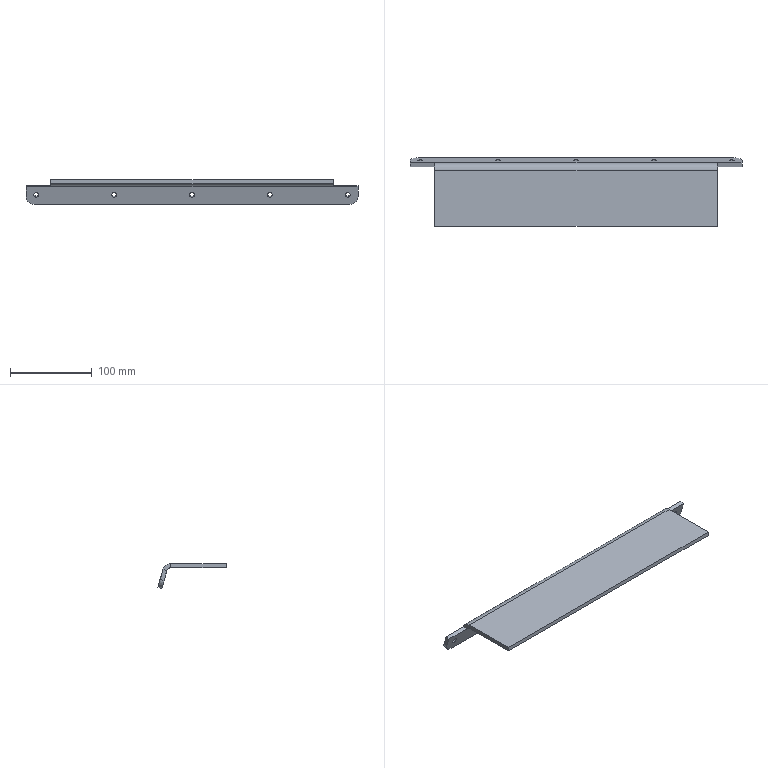Part | SolidWorks | features EdgeFlange 1, Fillet 1, FlatPattern 1, HoleWzd 1, SMBaseFlange 1, SheetMetal 1 | 1 solid | 38 faces | box 405 x 83.269 x 30.216 mm | volume 177655 mm3 | cylinder 14 | plane 14 | cone 10 | commonest cylinder face diameters 6 x10 20 x3 10 x1
STEP:
#1=CARTESIAN_POINT('',(-190.,43.243,-15.119));
#2=VERTEX_POINT('',#1);
#3=CARTESIAN_POINT('',(-190.,41.589,-9.351));
#4=VERTEX_POINT('',#3);
#5=CARTESIAN_POINT('',(-190.,42.416,-12.235));
#6=DIRECTION('',(0.,0.9613,0.2756));
#7=DIRECTION('',(0.,-0.2756,0.9613));
#8=AXIS2_PLACEMENT_3D('',#5,#6,#7);
#9=CIRCLE('',#8,3.);
#10=EDGE_CURVE('',#2,#4,#9,.T.);
#11=ORIENTED_EDGE('',*,*,#10,.F.);
#12=CARTESIAN_POINT('',(-190.,43.274,-15.136));
#13=VERTEX_POINT('',#12);
#14=CARTESIAN_POINT('',(-190.,43.274,-15.136));
#15=DIRECTION('',(0.,0.8746,-0.4848));
#16=VECTOR('',#15,1000.);
#17=LINE('',#14,#16);
#18=EDGE_CURVE('',#2,#13,#17,.T.);
#19=ORIENTED_EDGE('',*,*,#18,.T.);
#20=CARTESIAN_POINT('',(-190.,41.606,-9.32));
#21=VERTEX_POINT('',#20);
#22=CARTESIAN_POINT('',(-190.,42.44,-12.228));
#23=DIRECTION('',(0.,0.9613,0.2756));
#24=DIRECTION('',(0.,-0.2756,0.9613));
#25=AXIS2_PLACEMENT_3D('',#22,#23,#24);
#26=CIRCLE('',#25,3.025);
#27=EDGE_CURVE('',#13,#21,#26,.T.);
#28=ORIENTED_EDGE('',*,*,#27,.T.);
#29=CARTESIAN_POINT('',(-190.,41.606,-9.32));
#30=DIRECTION('',(0.,0.4848,0.8746));
#31=VECTOR('',#30,1000.);
#32=LINE('',#29,#31);
#33=EDGE_CURVE('',#4,#21,#32,.T.);
#34=ORIENTED_EDGE('',*,*,#33,.F.);
#35=EDGE_LOOP('',(#11,#19,#28,#34));
#36=FACE_OUTER_BOUND('',#35,.T.);
#37=CARTESIAN_POINT('',(-190.,42.44,-12.228));
#38=DIRECTION('',(0.,0.9613,0.2756));
#39=DIRECTION('',(0.,-0.2756,0.9613));
#40=AXIS2_PLACEMENT_3D('',#37,#38,#39);
#41=CONICAL_SURFACE('',#40,3.025,0.7854);
#42=ADVANCED_FACE('',(#36),#41,.F.);
#43=CARTESIAN_POINT('',(-190.,38.461,-16.49));
#44=VERTEX_POINT('',#43);
#45=CARTESIAN_POINT('',(-190.,36.807,-10.723));
#46=VERTEX_POINT('',#45);
#47=CARTESIAN_POINT('',(-190.,37.634,-13.606));
#48=DIRECTION('',(0.,0.9613,0.2756));
#49=DIRECTION('',(0.,-0.2756,0.9613));
#50=AXIS2_PLACEMENT_3D('',#47,#48,#49);
#51=CIRCLE('',#50,3.);
#52=EDGE_CURVE('',#44,#46,#51,.T.);
#53=ORIENTED_EDGE('',*,*,#52,.F.);
#54=CARTESIAN_POINT('',(-190.,43.267,-15.112));
#55=DIRECTION('',(0.,0.9613,0.2756));
#56=VECTOR('',#55,1000.);
#57=LINE('',#54,#56);
#58=EDGE_CURVE('',#44,#2,#57,.T.);
#59=ORIENTED_EDGE('',*,*,#58,.T.);
#60=ORIENTED_EDGE('',*,*,#10,.T.);
#61=CARTESIAN_POINT('',(-190.,41.613,-9.344));
#62=DIRECTION('',(0.,0.9613,0.2756));
#63=VECTOR('',#62,1000.);
#64=LINE('',#61,#63);
#65=EDGE_CURVE('',#46,#4,#64,.T.);
#66=ORIENTED_EDGE('',*,*,#65,.F.);
#67=EDGE_LOOP('',(#53,#59,#60,#66));
#68=FACE_OUTER_BOUND('',#67,.T.);
#69=CARTESIAN_POINT('',(-190.,42.44,-12.228));
#70=DIRECTION('',(0.,0.9613,0.2756));
#71=DIRECTION('',(0.,-0.2756,0.9613));
#72=AXIS2_PLACEMENT_3D('',#69,#70,#71);
#73=CYLINDRICAL_SURFACE('',#72,3.);
#74=ADVANCED_FACE('',(#68),#73,.F.);
#75=CARTESIAN_POINT('',(-95.,43.243,-15.119));
#76=VERTEX_POINT('',#75);
#77=CARTESIAN_POINT('',(-95.,41.589,-9.351));
#78=VERTEX_POINT('',#77);
#79=CARTESIAN_POINT('',(-95.,42.416,-12.235));
#80=DIRECTION('',(0.,0.9613,0.2756));
#81=DIRECTION('',(0.,-0.2756,0.9613));
#82=AXIS2_PLACEMENT_3D('',#79,#80,#81);
#83=CIRCLE('',#82,3.);
#84=EDGE_CURVE('',#76,#78,#83,.T.);
#85=ORIENTED_EDGE('',*,*,#84,.F.);
#86=CARTESIAN_POINT('',(-95.,43.274,-15.136));
#87=VERTEX_POINT('',#86);
#88=CARTESIAN_POINT('',(-95.,43.274,-15.136));
#89=DIRECTION('',(0.,0.8746,-0.4848));
#90=VECTOR('',#89,1000.);
#91=LINE('',#88,#90);
#92=EDGE_CURVE('',#76,#87,#91,.T.);
#93=ORIENTED_EDGE('',*,*,#92,.T.);
#94=CARTESIAN_POINT('',(-95.,41.606,-9.32));
#95=VERTEX_POINT('',#94);
#96=CARTESIAN_POINT('',(-95.,42.44,-12.228));
#97=DIRECTION('',(0.,0.9613,0.2756));
#98=DIRECTION('',(0.,-0.2756,0.9613));
#99=AXIS2_PLACEMENT_3D('',#96,#97,#98);
#100=CIRCLE('',#99,3.025);
#101=EDGE_CURVE('',#87,#95,#100,.T.);
#102=ORIENTED_EDGE('',*,*,#101,.T.);
#103=CARTESIAN_POINT('',(-95.,41.606,-9.32));
#104=DIRECTION('',(0.,0.4848,0.8746));
#105=VECTOR('',#104,1000.);
#106=LINE('',#103,#105);
#107=EDGE_CURVE('',#78,#95,#106,.T.);
#108=ORIENTED_EDGE('',*,*,#107,.F.);
#109=EDGE_LOOP('',(#85,#93,#102,#108));
#110=FACE_OUTER_BOUND('',#109,.T.);
#111=CARTESIAN_POINT('',(-95.,42.44,-12.228));
#112=DIRECTION('',(0.,0.9613,0.2756));
#113=DIRECTION('',(0.,-0.2756,0.9613));
#114=AXIS2_PLACEMENT_3D('',#111,#112,#113);
#115=CONICAL_SURFACE('',#114,3.025,0.7854);
#116=ADVANCED_FACE('',(#110),#115,.F.);
#117=CARTESIAN_POINT('',(-95.,38.461,-16.49));
#118=VERTEX_POINT('',#117);
#119=CARTESIAN_POINT('',(-95.,36.807,-10.723));
#120=VERTEX_POINT('',#119);
#121=CARTESIAN_POINT('',(-95.,37.634,-13.606));
#122=DIRECTION('',(0.,0.9613,0.2756));
#123=DIRECTION('',(0.,-0.2756,0.9613));
#124=AXIS2_PLACEMENT_3D('',#121,#122,#123);
#125=CIRCLE('',#124,3.);
#126=EDGE_CURVE('',#118,#120,#125,.T.);
#127=ORIENTED_EDGE('',*,*,#126,.F.);
#128=CARTESIAN_POINT('',(-95.,43.267,-15.112));
#129=DIRECTION('',(0.,0.9613,0.2756));
#130=VECTOR('',#129,1000.);
#131=LINE('',#128,#130);
#132=EDGE_CURVE('',#118,#76,#131,.T.);
#133=ORIENTED_EDGE('',*,*,#132,.T.);
#134=ORIENTED_EDGE('',*,*,#84,.T.);
#135=CARTESIAN_POINT('',(-95.,41.613,-9.344));
#136=DIRECTION('',(0.,0.9613,0.2756));
#137=VECTOR('',#136,1000.);
#138=LINE('',#135,#137);
#139=EDGE_CURVE('',#120,#78,#138,.T.);
#140=ORIENTED_EDGE('',*,*,#139,.F.);
#141=EDGE_LOOP('',(#127,#133,#134,#140));
#142=FACE_OUTER_BOUND('',#141,.T.);
#143=CARTESIAN_POINT('',(-95.,42.44,-12.228));
#144=DIRECTION('',(0.,0.9613,0.2756));
#145=DIRECTION('',(0.,-0.2756,0.9613));
#146=AXIS2_PLACEMENT_3D('',#143,#144,#145);
#147=CYLINDRICAL_SURFACE('',#146,3.);
#148=ADVANCED_FACE('',(#142),#147,.F.);
#149=CARTESIAN_POINT('',(0.,43.243,-15.119));
#150=VERTEX_POINT('',#149);
#151=CARTESIAN_POINT('',(0.,41.589,-9.351));
#152=VERTEX_POINT('',#151);
#153=CARTESIAN_POINT('',(0.,42.416,-12.235));
#154=DIRECTION('',(0.,0.9613,0.2756));
#155=DIRECTION('',(0.,-0.2756,0.9613));
#156=AXIS2_PLACEMENT_3D('',#153,#154,#155);
#157=CIRCLE('',#156,3.);
#158=EDGE_CURVE('',#150,#152,#157,.T.);
#159=ORIENTED_EDGE('',*,*,#158,.F.);
#160=CARTESIAN_POINT('',(0.,43.274,-15.136));
#161=VERTEX_POINT('',#160);
#162=CARTESIAN_POINT('',(0.,43.274,-15.136));
#163=DIRECTION('',(0.,0.8746,-0.4848));
#164=VECTOR('',#163,1000.);
#165=LINE('',#162,#164);
#166=EDGE_CURVE('',#150,#161,#165,.T.);
#167=ORIENTED_EDGE('',*,*,#166,.T.);
#168=CARTESIAN_POINT('',(0.,41.606,-9.32));
#169=VERTEX_POINT('',#168);
#170=CARTESIAN_POINT('',(0.,42.44,-12.228));
#171=DIRECTION('',(0.,0.9613,0.2756));
#172=DIRECTION('',(0.,-0.2756,0.9613));
#173=AXIS2_PLACEMENT_3D('',#170,#171,#172);
#174=CIRCLE('',#173,3.025);
#175=EDGE_CURVE('',#161,#169,#174,.T.);
#176=ORIENTED_EDGE('',*,*,#175,.T.);
#177=CARTESIAN_POINT('',(0.,41.606,-9.32));
#178=DIRECTION('',(0.,0.4848,0.8746));
#179=VECTOR('',#178,1000.);
#180=LINE('',#177,#179);
#181=EDGE_CURVE('',#152,#169,#180,.T.);
#182=ORIENTED_EDGE('',*,*,#181,.F.);
#183=EDGE_LOOP('',(#159,#167,#176,#182));
#184=FACE_OUTER_BOUND('',#183,.T.);
#185=CARTESIAN_POINT('',(0.,42.44,-12.228));
#186=DIRECTION('',(0.,0.9613,0.2756));
#187=DIRECTION('',(0.,-0.2756,0.9613));
#188=AXIS2_PLACEMENT_3D('',#185,#186,#187);
#189=CONICAL_SURFACE('',#188,3.025,0.7854);
#190=ADVANCED_FACE('',(#184),#189,.F.);
#191=CARTESIAN_POINT('',(0.,38.461,-16.49));
#192=VERTEX_POINT('',#191);
#193=CARTESIAN_POINT('',(0.,36.807,-10.723));
#194=VERTEX_POINT('',#193);
#195=CARTESIAN_POINT('',(0.,37.634,-13.606));
#196=DIRECTION('',(0.,0.9613,0.2756));
#197=DIRECTION('',(0.,-0.2756,0.9613));
#198=AXIS2_PLACEMENT_3D('',#195,#196,#197);
#199=CIRCLE('',#198,3.);
#200=EDGE_CURVE('',#192,#194,#199,.T.);
#201=ORIENTED_EDGE('',*,*,#200,.F.);
#202=CARTESIAN_POINT('',(0.,43.267,-15.112));
#203=DIRECTION('',(0.,0.9613,0.2756));
#204=VECTOR('',#203,1000.);
#205=LINE('',#202,#204);
#206=EDGE_CURVE('',#192,#150,#205,.T.);
#207=ORIENTED_EDGE('',*,*,#206,.T.);
#208=ORIENTED_EDGE('',*,*,#158,.T.);
#209=CARTESIAN_POINT('',(0.,41.613,-9.344));
#210=DIRECTION('',(0.,0.9613,0.2756));
#211=VECTOR('',#210,1000.);
#212=LINE('',#209,#211);
#213=EDGE_CURVE('',#194,#152,#212,.T.);
#214=ORIENTED_EDGE('',*,*,#213,.F.);
#215=EDGE_LOOP('',(#201,#207,#208,#214));
#216=FACE_OUTER_BOUND('',#215,.T.);
#217=CARTESIAN_POINT('',(0.,42.44,-12.228));
#218=DIRECTION('',(0.,0.9613,0.2756));
#219=DIRECTION('',(0.,-0.2756,0.9613));
#220=AXIS2_PLACEMENT_3D('',#217,#218,#219);
#221=CYLINDRICAL_SURFACE('',#220,3.);
#222=ADVANCED_FACE('',(#216),#221,.F.);
#223=CARTESIAN_POINT('',(95.,43.243,-15.119));
#224=VERTEX_POINT('',#223);
#225=CARTESIAN_POINT('',(95.,41.589,-9.351));
#226=VERTEX_POINT('',#225);
#227=CARTESIAN_POINT('',(95.,42.416,-12.235));
#228=DIRECTION('',(0.,0.9613,0.2756));
#229=DIRECTION('',(0.,-0.2756,0.9613));
#230=AXIS2_PLACEMENT_3D('',#227,#228,#229);
#231=CIRCLE('',#230,3.);
#232=EDGE_CURVE('',#224,#226,#231,.T.);
#233=ORIENTED_EDGE('',*,*,#232,.F.);
#234=CARTESIAN_POINT('',(95.,43.274,-15.136));
#235=VERTEX_POINT('',#234);
#236=CARTESIAN_POINT('',(95.,43.274,-15.136));
#237=DIRECTION('',(0.,0.8746,-0.4848));
#238=VECTOR('',#237,1000.);
#239=LINE('',#236,#238);
#240=EDGE_CURVE('',#224,#235,#239,.T.);
#241=ORIENTED_EDGE('',*,*,#240,.T.);
#242=CARTESIAN_POINT('',(95.,41.606,-9.32));
#243=VERTEX_POINT('',#242);
#244=CARTESIAN_POINT('',(95.,42.44,-12.228));
#245=DIRECTION('',(0.,0.9613,0.2756));
#246=DIRECTION('',(0.,-0.2756,0.9613));
#247=AXIS2_PLACEMENT_3D('',#244,#245,#246);
#248=CIRCLE('',#247,3.025);
#249=EDGE_CURVE('',#235,#243,#248,.T.);
#250=ORIENTED_EDGE('',*,*,#249,.T.);
#251=CARTESIAN_POINT('',(95.,41.606,-9.32));
#252=DIRECTION('',(0.,0.4848,0.8746));
#253=VECTOR('',#252,1000.);
#254=LINE('',#251,#253);
#255=EDGE_CURVE('',#226,#243,#254,.T.);
#256=ORIENTED_EDGE('',*,*,#255,.F.);
#257=EDGE_LOOP('',(#233,#241,#250,#256));
#258=FACE_OUTER_BOUND('',#257,.T.);
#259=CARTESIAN_POINT('',(95.,42.44,-12.228));
#260=DIRECTION('',(0.,0.9613,0.2756));
#261=DIRECTION('',(0.,-0.2756,0.9613));
#262=AXIS2_PLACEMENT_3D('',#259,#260,#261);
#263=CONICAL_SURFACE('',#262,3.025,0.7854);
#264=ADVANCED_FACE('',(#258),#263,.F.);
#265=CARTESIAN_POINT('',(95.,38.461,-16.49));
#266=VERTEX_POINT('',#265);
#267=CARTESIAN_POINT('',(95.,36.807,-10.723));
#268=VERTEX_POINT('',#267);
#269=CARTESIAN_POINT('',(95.,37.634,-13.606));
#270=DIRECTION('',(0.,0.9613,0.2756));
#271=DIRECTION('',(0.,-0.2756,0.9613));
#272=AXIS2_PLACEMENT_3D('',#269,#270,#271);
#273=CIRCLE('',#272,3.);
#274=EDGE_CURVE('',#266,#268,#273,.T.);
#275=ORIENTED_EDGE('',*,*,#274,.F.);
#276=CARTESIAN_POINT('',(95.,43.267,-15.112));
#277=DIRECTION('',(0.,0.9613,0.2756));
#278=VECTOR('',#277,1000.);
#279=LINE('',#276,#278);
#280=EDGE_CURVE('',#266,#224,#279,.T.);
#281=ORIENTED_EDGE('',*,*,#280,.T.);
#282=ORIENTED_EDGE('',*,*,#232,.T.);
#283=CARTESIAN_POINT('',(95.,41.613,-9.344));
#284=DIRECTION('',(0.,0.9613,0.2756));
#285=VECTOR('',#284,1000.);
#286=LINE('',#283,#285);
#287=EDGE_CURVE('',#268,#226,#286,.T.);
#288=ORIENTED_EDGE('',*,*,#287,.F.);
#289=EDGE_LOOP('',(#275,#281,#282,#288));
#290=FACE_OUTER_BOUND('',#289,.T.);
#291=CARTESIAN_POINT('',(95.,42.44,-12.228));
#292=DIRECTION('',(0.,0.9613,0.2756));
#293=DIRECTION('',(0.,-0.2756,0.9613));
#294=AXIS2_PLACEMENT_3D('',#291,#292,#293);
#295=CYLINDRICAL_SURFACE('',#294,3.);
#296=ADVANCED_FACE('',(#290),#295,.F.);
#297=CARTESIAN_POINT('',(190.,43.243,-15.119));
#298=VERTEX_POINT('',#297);
#299=CARTESIAN_POINT('',(190.,41.589,-9.351));
#300=VERTEX_POINT('',#299);
#301=CARTESIAN_POINT('',(190.,42.416,-12.235));
#302=DIRECTION('',(0.,0.9613,0.2756));
#303=DIRECTION('',(0.,-0.2756,0.9613));
#304=AXIS2_PLACEMENT_3D('',#301,#302,#303);
#305=CIRCLE('',#304,3.);
#306=EDGE_CURVE('',#298,#300,#305,.T.);
#307=ORIENTED_EDGE('',*,*,#306,.F.);
#308=CARTESIAN_POINT('',(190.,43.274,-15.136));
#309=VERTEX_POINT('',#308);
#310=CARTESIAN_POINT('',(190.,43.274,-15.136));
#311=DIRECTION('',(0.,0.8746,-0.4848));
#312=VECTOR('',#311,1000.);
#313=LINE('',#310,#312);
#314=EDGE_CURVE('',#298,#309,#313,.T.);
#315=ORIENTED_EDGE('',*,*,#314,.T.);
#316=CARTESIAN_POINT('',(190.,41.606,-9.32));
#317=VERTEX_POINT('',#316);
#318=CARTESIAN_POINT('',(190.,42.44,-12.228));
#319=DIRECTION('',(0.,0.9613,0.2756));
#320=DIRECTION('',(0.,-0.2756,0.9613));
#321=AXIS2_PLACEMENT_3D('',#318,#319,#320);
#322=CIRCLE('',#321,3.025);
#323=EDGE_CURVE('',#309,#317,#322,.T.);
#324=ORIENTED_EDGE('',*,*,#323,.T.);
#325=CARTESIAN_POINT('',(190.,41.606,-9.32));
#326=DIRECTION('',(0.,0.4848,0.8746));
#327=VECTOR('',#326,1000.);
#328=LINE('',#325,#327);
#329=EDGE_CURVE('',#300,#317,#328,.T.);
#330=ORIENTED_EDGE('',*,*,#329,.F.);
#331=EDGE_LOOP('',(#307,#315,#324,#330));
#332=FACE_OUTER_BOUND('',#331,.T.);
#333=CARTESIAN_POINT('',(190.,42.44,-12.228));
#334=DIRECTION('',(0.,0.9613,0.2756));
#335=DIRECTION('',(0.,-0.2756,0.9613));
#336=AXIS2_PLACEMENT_3D('',#333,#334,#335);
#337=CONICAL_SURFACE('',#336,3.025,0.7854);
#338=ADVANCED_FACE('',(#332),#337,.F.);
#339=CARTESIAN_POINT('',(190.,38.461,-16.49));
#340=VERTEX_POINT('',#339);
#341=CARTESIAN_POINT('',(190.,36.807,-10.723));
#342=VERTEX_POINT('',#341);
#343=CARTESIAN_POINT('',(190.,37.634,-13.606));
#344=DIRECTION('',(0.,0.9613,0.2756));
#345=DIRECTION('',(0.,-0.2756,0.9613));
#346=AXIS2_PLACEMENT_3D('',#343,#344,#345);
#347=CIRCLE('',#346,3.);
#348=EDGE_CURVE('',#340,#342,#347,.T.);
#349=ORIENTED_EDGE('',*,*,#348,.F.);
#350=CARTESIAN_POINT('',(190.,43.267,-15.112));
#351=DIRECTION('',(0.,0.9613,0.2756));
#352=VECTOR('',#351,1000.);
#353=LINE('',#350,#352);
#354=EDGE_CURVE('',#340,#298,#353,.T.);
#355=ORIENTED_EDGE('',*,*,#354,.T.);
#356=ORIENTED_EDGE('',*,*,#306,.T.);
#357=CARTESIAN_POINT('',(190.,41.613,-9.344));
#358=DIRECTION('',(0.,0.9613,0.2756));
#359=VECTOR('',#358,1000.);
#360=LINE('',#357,#359);
#361=EDGE_CURVE('',#342,#300,#360,.T.);
#362=ORIENTED_EDGE('',*,*,#361,.F.);
#363=EDGE_LOOP('',(#349,#355,#356,#362));
#364=FACE_OUTER_BOUND('',#363,.T.);
#365=CARTESIAN_POINT('',(190.,42.44,-12.228));
#366=DIRECTION('',(0.,0.9613,0.2756));
#367=DIRECTION('',(0.,-0.2756,0.9613));
#368=AXIS2_PLACEMENT_3D('',#365,#366,#367);
#369=CYLINDRICAL_SURFACE('',#368,3.);
#370=ADVANCED_FACE('',(#364),#369,.F.);
#371=CARTESIAN_POINT('',(172.5,29.964,0.));
#372=VERTEX_POINT('',#371);
#373=CARTESIAN_POINT('',(172.5,29.964,5.));
#374=VERTEX_POINT('',#373);
#375=CARTESIAN_POINT('',(172.5,29.964,0.));
#376=DIRECTION('',(0.,0.,1.));
#377=VECTOR('',#376,1000.);
#378=LINE('',#375,#377);
#379=EDGE_CURVE('',#372,#374,#378,.T.);
#380=ORIENTED_EDGE('',*,*,#379,.T.);
#381=CARTESIAN_POINT('',(172.5,-37.5,5.));
#382=VERTEX_POINT('',#381);
#383=CARTESIAN_POINT('',(172.5,37.5,5.));
#384=DIRECTION('',(0.,1.,0.));
#385=VECTOR('',#384,1000.);
#386=LINE('',#383,#385);
#387=EDGE_CURVE('',#382,#374,#386,.T.);
#388=ORIENTED_EDGE('',*,*,#387,.F.);
#389=CARTESIAN_POINT('',(172.5,-37.5,0.));
#390=VERTEX_POINT('',#389);
#391=CARTESIAN_POINT('',(172.5,-37.5,5.));
#392=DIRECTION('',(0.,0.,-1.));
#393=VECTOR('',#392,1000.);
#394=LINE('',#391,#393);
#395=EDGE_CURVE('',#382,#390,#394,.T.);
#396=ORIENTED_EDGE('',*,*,#395,.T.);
#397=CARTESIAN_POINT('',(172.5,37.5,0.));
#398=DIRECTION('',(0.,1.,0.));
#399=VECTOR('',#398,1000.);
#400=LINE('',#397,#399);
#401=EDGE_CURVE('',#390,#372,#400,.T.);
#402=ORIENTED_EDGE('',*,*,#401,.T.);
#403=EDGE_LOOP('',(#380,#388,#396,#402));
#404=FACE_OUTER_BOUND('',#403,.T.);
#405=CARTESIAN_POINT('',(172.5,37.5,5.));
#406=DIRECTION('',(-1.,0.,0.));
#407=DIRECTION('',(0.,-1.,0.));
#408=AXIS2_PLACEMENT_3D('',#405,#406,#407);
#409=PLANE('',#408);
#410=ADVANCED_FACE('',(#404),#409,.F.);
#411=CARTESIAN_POINT('',(-172.5,29.964,0.));
#412=VERTEX_POINT('',#411);
#413=CARTESIAN_POINT('',(-172.5,29.964,5.));
#414=VERTEX_POINT('',#413);
#415=CARTESIAN_POINT('',(-172.5,29.964,0.));
#416=DIRECTION('',(0.,0.,1.));
#417=VECTOR('',#416,1000.);
#418=LINE('',#415,#417);
#419=EDGE_CURVE('',#412,#414,#418,.T.);
#420=ORIENTED_EDGE('',*,*,#419,.F.);
#421=CARTESIAN_POINT('',(-172.5,-37.5,0.));
#422=VERTEX_POINT('',#421);
#423=CARTESIAN_POINT('',(-172.5,37.5,0.));
#424=DIRECTION('',(0.,-1.,0.));
#425=VECTOR('',#424,1000.);
#426=LINE('',#423,#425);
#427=EDGE_CURVE('',#412,#422,#426,.T.);
#428=ORIENTED_EDGE('',*,*,#427,.T.);
#429=CARTESIAN_POINT('',(-172.5,-37.5,5.));
#430=VERTEX_POINT('',#429);
#431=CARTESIAN_POINT('',(-172.5,-37.5,5.));
#432=DIRECTION('',(0.,0.,-1.));
#433=VECTOR('',#432,1000.);
#434=LINE('',#431,#433);
#435=EDGE_CURVE('',#430,#422,#434,.T.);
#436=ORIENTED_EDGE('',*,*,#435,.F.);
#437=CARTESIAN_POINT('',(-172.5,37.5,5.));
#438=DIRECTION('',(0.,-1.,0.));
#439=VECTOR('',#438,1000.);
#440=LINE('',#437,#439);
#441=EDGE_CURVE('',#414,#430,#440,.T.);
#442=ORIENTED_EDGE('',*,*,#441,.F.);
#443=EDGE_LOOP('',(#420,#428,#436,#442));
#444=FACE_OUTER_BOUND('',#443,.T.);
#445=CARTESIAN_POINT('',(-172.5,37.5,5.));
#446=DIRECTION('',(1.,0.,0.));
#447=DIRECTION('',(0.,0.,-1.));
#448=AXIS2_PLACEMENT_3D('',#445,#446,#447);
#449=PLANE('',#448);
#450=ADVANCED_FACE('',(#444),#449,.F.);
#451=ORIENTED_EDGE('',*,*,#387,.T.);
#452=CARTESIAN_POINT('',(172.5,29.964,5.));
#453=DIRECTION('',(-1.,0.,0.));
#454=VECTOR('',#453,1000.);
#455=LINE('',#452,#454);
#456=EDGE_CURVE('',#374,#414,#455,.T.);
#457=ORIENTED_EDGE('',*,*,#456,.T.);
#458=ORIENTED_EDGE('',*,*,#441,.T.);
#459=CARTESIAN_POINT('',(-172.5,-37.5,5.));
#460=DIRECTION('',(1.,0.,0.));
#461=VECTOR('',#460,1000.);
#462=LINE('',#459,#461);
#463=EDGE_CURVE('',#430,#382,#462,.T.);
#464=ORIENTED_EDGE('',*,*,#463,.T.);
#465=EDGE_LOOP('',(#451,#457,#458,#464));
#466=FACE_OUTER_BOUND('',#465,.T.);
#467=CARTESIAN_POINT('',(0.,0.,5.));
#468=DIRECTION('',(0.,0.,1.));
#469=DIRECTION('',(1.,0.,0.));
#470=AXIS2_PLACEMENT_3D('',#467,#468,#469);
#471=PLANE('',#470);
#472=ADVANCED_FACE('',(#466),#471,.T.);
#473=CARTESIAN_POINT('',(172.5,29.964,0.));
#474=DIRECTION('',(-1.,0.,0.));
#475=VECTOR('',#474,1000.);
#476=LINE('',#473,#475);
#477=EDGE_CURVE('',#372,#412,#476,.T.);
#478=ORIENTED_EDGE('',*,*,#477,.F.);
#479=ORIENTED_EDGE('',*,*,#401,.F.);
#480=CARTESIAN_POINT('',(-172.5,-37.5,0.));
#481=DIRECTION('',(1.,0.,0.));
#482=VECTOR('',#481,1000.);
#483=LINE('',#480,#482);
#484=EDGE_CURVE('',#422,#390,#483,.T.);
#485=ORIENTED_EDGE('',*,*,#484,.F.);
#486=ORIENTED_EDGE('',*,*,#427,.F.);
#487=EDGE_LOOP('',(#478,#479,#485,#486));
#488=FACE_OUTER_BOUND('',#487,.T.);
#489=CARTESIAN_POINT('',(0.,0.,0.));
#490=DIRECTION('',(0.,0.,1.));
#491=DIRECTION('',(1.,0.,0.));
#492=AXIS2_PLACEMENT_3D('',#489,#490,#491);
#493=PLANE('',#492);
#494=ADVANCED_FACE('',(#488),#493,.F.);
#495=ORIENTED_EDGE('',*,*,#484,.T.);
#496=ORIENTED_EDGE('',*,*,#395,.F.);
#497=ORIENTED_EDGE('',*,*,#463,.F.);
#498=ORIENTED_EDGE('',*,*,#435,.T.);
#499=EDGE_LOOP('',(#495,#496,#497,#498));
#500=FACE_OUTER_BOUND('',#499,.T.);
#501=CARTESIAN_POINT('',(-172.5,-37.5,5.));
#502=DIRECTION('',(0.,1.,0.));
#503=DIRECTION('',(0.,0.,1.));
#504=AXIS2_PLACEMENT_3D('',#501,#502,#503);
#505=PLANE('',#504);
#506=ADVANCED_FACE('',(#500),#505,.F.);
#507=CARTESIAN_POINT('',(-172.5,34.771,-3.622));
#508=VERTEX_POINT('',#507);
#509=CARTESIAN_POINT('',(-172.5,39.577,-2.244));
#510=VERTEX_POINT('',#509);
#511=CARTESIAN_POINT('',(-172.5,34.771,-3.622));
#512=DIRECTION('',(0.,0.9613,0.2756));
#513=VECTOR('',#512,1000.);
#514=LINE('',#511,#513);
#515=EDGE_CURVE('',#508,#510,#514,.T.);
#516=ORIENTED_EDGE('',*,*,#515,.F.);
#517=CARTESIAN_POINT('',(-172.5,29.964,-5.));
#518=DIRECTION('',(-1.,0.,0.));
#519=DIRECTION('',(0.,0.,-1.));
#520=AXIS2_PLACEMENT_3D('',#517,#518,#519);
#521=CIRCLE('',#520,5.);
#522=EDGE_CURVE('',#412,#508,#521,.T.);
#523=ORIENTED_EDGE('',*,*,#522,.F.);
#524=ORIENTED_EDGE('',*,*,#419,.T.);
#525=CARTESIAN_POINT('',(-172.5,29.964,-5.));
#526=DIRECTION('',(-1.,0.,0.));
#527=DIRECTION('',(0.,0.,-1.));
#528=AXIS2_PLACEMENT_3D('',#525,#526,#527);
#529=CIRCLE('',#528,10.);
#530=EDGE_CURVE('',#414,#510,#529,.T.);
#531=ORIENTED_EDGE('',*,*,#530,.T.);
#532=EDGE_LOOP('',(#516,#523,#524,#531));
#533=FACE_OUTER_BOUND('',#532,.T.);
#534=CARTESIAN_POINT('',(-172.5,29.964,-5.));
#535=DIRECTION('',(-1.,0.,0.));
#536=DIRECTION('',(0.,0.,1.));
#537=AXIS2_PLACEMENT_3D('',#534,#535,#536);
#538=PLANE('',#537);
#539=ADVANCED_FACE('',(#533),#538,.T.);
#540=CARTESIAN_POINT('',(172.5,34.771,-3.622));
#541=VERTEX_POINT('',#540);
#542=CARTESIAN_POINT('',(172.5,29.964,-5.));
#543=DIRECTION('',(1.,0.,0.));
#544=DIRECTION('',(0.,0.,-1.));
#545=AXIS2_PLACEMENT_3D('',#542,#543,#544);
#546=CIRCLE('',#545,5.);
#547=EDGE_CURVE('',#541,#372,#546,.T.);
#548=ORIENTED_EDGE('',*,*,#547,.F.);
#549=CARTESIAN_POINT('',(172.5,39.577,-2.244));
#550=VERTEX_POINT('',#549);
#551=CARTESIAN_POINT('',(172.5,34.771,-3.622));
#552=DIRECTION('',(0.,0.9613,0.2756));
#553=VECTOR('',#552,1000.);
#554=LINE('',#551,#553);
#555=EDGE_CURVE('',#541,#550,#554,.T.);
#556=ORIENTED_EDGE('',*,*,#555,.T.);
#557=CARTESIAN_POINT('',(172.5,29.964,-5.));
#558=DIRECTION('',(1.,0.,0.));
#559=DIRECTION('',(0.,0.,-1.));
#560=AXIS2_PLACEMENT_3D('',#557,#558,#559);
#561=CIRCLE('',#560,10.);
#562=EDGE_CURVE('',#550,#374,#561,.T.);
#563=ORIENTED_EDGE('',*,*,#562,.T.);
#564=ORIENTED_EDGE('',*,*,#379,.F.);
#565=EDGE_LOOP('',(#548,#556,#563,#564));
#566=FACE_OUTER_BOUND('',#565,.T.);
#567=CARTESIAN_POINT('',(172.5,29.964,-5.));
#568=DIRECTION('',(-1.,0.,0.));
#569=DIRECTION('',(0.,0.,1.));
#570=AXIS2_PLACEMENT_3D('',#567,#568,#569);
#571=PLANE('',#570);
#572=ADVANCED_FACE('',(#566),#571,.F.);
#573=ORIENTED_EDGE('',*,*,#456,.F.);
#574=ORIENTED_EDGE('',*,*,#562,.F.);
#575=CARTESIAN_POINT('',(172.5,39.577,-2.244));
#576=DIRECTION('',(1.,0.,0.));
#577=VECTOR('',#576,1000.);
#578=LINE('',#575,#577);
#579=EDGE_CURVE('',#510,#550,#578,.T.);
#580=ORIENTED_EDGE('',*,*,#579,.F.);
#581=ORIENTED_EDGE('',*,*,#530,.F.);
#582=EDGE_LOOP('',(#573,#574,#580,#581));
#583=FACE_OUTER_BOUND('',#582,.T.);
#584=CARTESIAN_POINT('',(172.5,29.964,-5.));
#585=DIRECTION('',(1.,0.,0.));
#586=DIRECTION('',(0.,0.9613,0.2756));
#587=AXIS2_PLACEMENT_3D('',#584,#585,#586);
#588=CYLINDRICAL_SURFACE('',#587,10.);
#589=ADVANCED_FACE('',(#583),#588,.T.);
#590=ORIENTED_EDGE('',*,*,#477,.T.);
#591=ORIENTED_EDGE('',*,*,#522,.T.);
#592=CARTESIAN_POINT('',(172.5,34.771,-3.622));
#593=DIRECTION('',(1.,0.,0.));
#594=VECTOR('',#593,1000.);
#595=LINE('',#592,#594);
#596=EDGE_CURVE('',#508,#541,#595,.T.);
#597=ORIENTED_EDGE('',*,*,#596,.T.);
#598=ORIENTED_EDGE('',*,*,#547,.T.);
#599=EDGE_LOOP('',(#590,#591,#597,#598));
#600=FACE_OUTER_BOUND('',#599,.T.);
#601=CARTESIAN_POINT('',(172.5,29.964,-5.));
#602=DIRECTION('',(1.,0.,0.));
#603=DIRECTION('',(0.,0.9613,0.2756));
#604=AXIS2_PLACEMENT_3D('',#601,#602,#603);
#605=CYLINDRICAL_SURFACE('',#604,5.);
#606=ADVANCED_FACE('',(#600),#605,.F.);
#607=ORIENTED_EDGE('',*,*,#555,.F.);
#608=CARTESIAN_POINT('',(202.5,34.771,-3.622));
#609=VERTEX_POINT('',#608);
#610=CARTESIAN_POINT('',(-202.5,34.771,-3.622));
#611=DIRECTION('',(1.,0.,0.));
#612=VECTOR('',#611,1000.);
#613=LINE('',#610,#612);
#614=EDGE_CURVE('',#541,#609,#613,.T.);
#615=ORIENTED_EDGE('',*,*,#614,.T.);
#616=CARTESIAN_POINT('',(202.5,39.577,-2.244));
#617=VERTEX_POINT('',#616);
#618=CARTESIAN_POINT('',(202.5,34.771,-3.622));
#619=DIRECTION('',(0.,0.9613,0.2756));
#620=VECTOR('',#619,1000.);
#621=LINE('',#618,#620);
#622=EDGE_CURVE('',#609,#617,#621,.T.);
#623=ORIENTED_EDGE('',*,*,#622,.T.);
#624=CARTESIAN_POINT('',(0.,39.577,-2.244));
#625=DIRECTION('',(1.,0.,0.));
#626=VECTOR('',#625,1000.);
#627=LINE('',#624,#626);
#628=EDGE_CURVE('',#550,#617,#627,.T.);
#629=ORIENTED_EDGE('',*,*,#628,.F.);
#630=EDGE_LOOP('',(#607,#615,#623,#629));
#631=FACE_OUTER_BOUND('',#630,.T.);
#632=CARTESIAN_POINT('',(-202.5,34.771,-3.622));
#633=DIRECTION('',(0.,-0.2756,0.9613));
#634=DIRECTION('',(0.,-0.9613,-0.2756));
#635=AXIS2_PLACEMENT_3D('',#632,#633,#634);
#636=PLANE('',#635);
#637=ADVANCED_FACE('',(#631),#636,.T.);
#638=CARTESIAN_POINT('',(202.5,38.206,-15.603));
#639=VERTEX_POINT('',#638);
#640=CARTESIAN_POINT('',(202.5,30.883,9.936));
#641=DIRECTION('',(0.,-0.2756,0.9613));
#642=VECTOR('',#641,1000.);
#643=LINE('',#640,#642);
#644=EDGE_CURVE('',#639,#609,#643,.T.);
#645=ORIENTED_EDGE('',*,*,#644,.F.);
#646=CARTESIAN_POINT('',(202.5,43.013,-14.225));
#647=VERTEX_POINT('',#646);
#648=CARTESIAN_POINT('',(202.5,43.013,-14.225));
#649=DIRECTION('',(0.,0.9613,0.2756));
#650=VECTOR('',#649,1000.);
#651=LINE('',#648,#650);
#652=EDGE_CURVE('',#639,#647,#651,.T.);
#653=ORIENTED_EDGE('',*,*,#652,.T.);
#654=CARTESIAN_POINT('',(202.5,38.539,1.378));
#655=DIRECTION('',(0.,-0.2756,0.9613));
#656=VECTOR('',#655,1000.);
#657=LINE('',#654,#656);
#658=EDGE_CURVE('',#647,#617,#657,.T.);
#659=ORIENTED_EDGE('',*,*,#658,.T.);
#660=ORIENTED_EDGE('',*,*,#622,.F.);
#661=EDGE_LOOP('',(#645,#653,#659,#660));
#662=FACE_OUTER_BOUND('',#661,.T.);
#663=CARTESIAN_POINT('',(202.5,38.539,1.378));
#664=DIRECTION('',(1.,0.,0.));
#665=DIRECTION('',(0.,0.,-1.));
#666=AXIS2_PLACEMENT_3D('',#663,#664,#665);
#667=PLANE('',#666);
#668=ADVANCED_FACE('',(#662),#667,.T.);
#669=CARTESIAN_POINT('',(-202.5,39.577,-2.244));
#670=VERTEX_POINT('',#669);
#671=CARTESIAN_POINT('',(-202.5,43.013,-14.225));
#672=VERTEX_POINT('',#671);
#673=CARTESIAN_POINT('',(-202.5,45.769,-23.838));
#674=DIRECTION('',(0.,0.2756,-0.9613));
#675=VECTOR('',#674,1000.);
#676=LINE('',#673,#675);
#677=EDGE_CURVE('',#670,#672,#676,.T.);
#678=ORIENTED_EDGE('',*,*,#677,.T.);
#679=CARTESIAN_POINT('',(-202.5,38.206,-15.603));
#680=VERTEX_POINT('',#679);
#681=CARTESIAN_POINT('',(-202.5,43.013,-14.225));
#682=DIRECTION('',(0.,-0.9613,-0.2756));
#683=VECTOR('',#682,1000.);
#684=LINE('',#681,#683);
#685=EDGE_CURVE('',#672,#680,#684,.T.);
#686=ORIENTED_EDGE('',*,*,#685,.T.);
#687=CARTESIAN_POINT('',(-202.5,34.771,-3.622));
#688=VERTEX_POINT('',#687);
#689=CARTESIAN_POINT('',(-202.5,30.883,9.936));
#690=DIRECTION('',(0.,0.2756,-0.9613));
#691=VECTOR('',#690,1000.);
#692=LINE('',#689,#691);
#693=EDGE_CURVE('',#688,#680,#692,.T.);
#694=ORIENTED_EDGE('',*,*,#693,.F.);
#695=CARTESIAN_POINT('',(-202.5,39.577,-2.244));
#696=DIRECTION('',(0.,0.9613,0.2756));
#697=VECTOR('',#696,1000.);
#698=LINE('',#695,#697);
#699=EDGE_CURVE('',#688,#670,#698,.T.);
#700=ORIENTED_EDGE('',*,*,#699,.T.);
#701=EDGE_LOOP('',(#678,#686,#694,#700));
#702=FACE_OUTER_BOUND('',#701,.T.);
#703=CARTESIAN_POINT('',(-202.5,45.769,-23.838));
#704=DIRECTION('',(-1.,0.,0.));
#705=DIRECTION('',(0.,0.,1.));
#706=AXIS2_PLACEMENT_3D('',#703,#704,#705);
#707=PLANE('',#706);
#708=ADVANCED_FACE('',(#702),#707,.T.);
#709=CARTESIAN_POINT('',(-190.,42.44,-12.228));
#710=DIRECTION('',(0.,0.9613,0.2756));
#711=DIRECTION('',(0.,-0.2756,0.9613));
#712=AXIS2_PLACEMENT_3D('',#709,#710,#711);
#713=CIRCLE('',#712,3.025);
#714=EDGE_CURVE('',#21,#13,#713,.T.);
#715=ORIENTED_EDGE('',*,*,#714,.F.);
#716=ORIENTED_EDGE('',*,*,#27,.F.);
#717=EDGE_LOOP('',(#715,#716));
#718=FACE_BOUND('',#717,.T.);
#719=CARTESIAN_POINT('',(-95.,42.44,-12.228));
#720=DIRECTION('',(0.,0.9613,0.2756));
#721=DIRECTION('',(0.,-0.2756,0.9613));
#722=AXIS2_PLACEMENT_3D('',#719,#720,#721);
#723=CIRCLE('',#722,3.025);
#724=EDGE_CURVE('',#95,#87,#723,.T.);
#725=ORIENTED_EDGE('',*,*,#724,.F.);
#726=ORIENTED_EDGE('',*,*,#101,.F.);
#727=EDGE_LOOP('',(#725,#726));
#728=FACE_BOUND('',#727,.T.);
#729=CARTESIAN_POINT('',(0.,42.44,-12.228));
#730=DIRECTION('',(0.,0.9613,0.2756));
#731=DIRECTION('',(0.,-0.2756,0.9613));
#732=AXIS2_PLACEMENT_3D('',#729,#730,#731);
#733=CIRCLE('',#732,3.025);
#734=EDGE_CURVE('',#169,#161,#733,.T.);
#735=ORIENTED_EDGE('',*,*,#734,.F.);
#736=ORIENTED_EDGE('',*,*,#175,.F.);
#737=EDGE_LOOP('',(#735,#736));
#738=FACE_BOUND('',#737,.T.);
#739=CARTESIAN_POINT('',(95.,42.44,-12.228));
#740=DIRECTION('',(0.,0.9613,0.2756));
#741=DIRECTION('',(0.,-0.2756,0.9613));
#742=AXIS2_PLACEMENT_3D('',#739,#740,#741);
#743=CIRCLE('',#742,3.025);
#744=EDGE_CURVE('',#243,#235,#743,.T.);
#745=ORIENTED_EDGE('',*,*,#744,.F.);
#746=ORIENTED_EDGE('',*,*,#249,.F.);
#747=EDGE_LOOP('',(#745,#746));
#748=FACE_BOUND('',#747,.T.);
#749=CARTESIAN_POINT('',(190.,42.44,-12.228));
#750=DIRECTION('',(0.,0.9613,0.2756));
#751=DIRECTION('',(0.,-0.2756,0.9613));
#752=AXIS2_PLACEMENT_3D('',#749,#750,#751);
#753=CIRCLE('',#752,3.025);
#754=EDGE_CURVE('',#317,#309,#753,.T.);
#755=ORIENTED_EDGE('',*,*,#754,.F.);
#756=ORIENTED_EDGE('',*,*,#323,.F.);
#757=EDGE_LOOP('',(#755,#756));
#758=FACE_BOUND('',#757,.T.);
#759=ORIENTED_EDGE('',*,*,#658,.F.);
#760=CARTESIAN_POINT('',(192.5,45.769,-23.838));
#761=VERTEX_POINT('',#760);
#762=CARTESIAN_POINT('',(192.5,43.013,-14.225));
#763=DIRECTION('',(0.,0.9613,0.2756));
#764=DIRECTION('',(0.,-0.2756,0.9613));
#765=AXIS2_PLACEMENT_3D('',#762,#763,#764);
#766=CIRCLE('',#765,10.);
#767=EDGE_CURVE('',#647,#761,#766,.T.);
#768=ORIENTED_EDGE('',*,*,#767,.T.);
#769=CARTESIAN_POINT('',(-192.5,45.769,-23.838));
#770=VERTEX_POINT('',#769);
#771=CARTESIAN_POINT('',(202.5,45.769,-23.838));
#772=DIRECTION('',(1.,0.,0.));
#773=VECTOR('',#772,1000.);
#774=LINE('',#771,#773);
#775=EDGE_CURVE('',#770,#761,#774,.T.);
#776=ORIENTED_EDGE('',*,*,#775,.F.);
#777=CARTESIAN_POINT('',(-192.5,43.013,-14.225));
#778=DIRECTION('',(0.,0.9613,0.2756));
#779=DIRECTION('',(0.,-0.2756,0.9613));
#780=AXIS2_PLACEMENT_3D('',#777,#778,#779);
#781=CIRCLE('',#780,10.);
#782=EDGE_CURVE('',#770,#672,#781,.T.);
#783=ORIENTED_EDGE('',*,*,#782,.T.);
#784=ORIENTED_EDGE('',*,*,#677,.F.);
#785=CARTESIAN_POINT('',(0.,39.577,-2.244));
#786=DIRECTION('',(1.,0.,0.));
#787=VECTOR('',#786,1000.);
#788=LINE('',#785,#787);
#789=EDGE_CURVE('',#670,#510,#788,.T.);
#790=ORIENTED_EDGE('',*,*,#789,.T.);
#791=ORIENTED_EDGE('',*,*,#579,.T.);
#792=ORIENTED_EDGE('',*,*,#628,.T.);
#793=EDGE_LOOP('',(#759,#768,#776,#783,#784,#790,#791,#792));
#794=FACE_OUTER_BOUND('',#793,.T.);
#795=CARTESIAN_POINT('',(0.,35.689,11.314));
#796=DIRECTION('',(0.,0.9613,0.2756));
#797=DIRECTION('',(0.,-0.2756,0.9613));
#798=AXIS2_PLACEMENT_3D('',#795,#796,#797);
#799=PLANE('',#798);
#800=ADVANCED_FACE('',(#718,#728,#738,#748,#758,#794),#799,.T.);
#801=CARTESIAN_POINT('',(-190.,37.634,-13.606));
#802=DIRECTION('',(0.,0.9613,0.2756));
#803=DIRECTION('',(0.,-0.2756,0.9613));
#804=AXIS2_PLACEMENT_3D('',#801,#802,#803);
#805=CIRCLE('',#804,3.);
#806=EDGE_CURVE('',#46,#44,#805,.T.);
#807=ORIENTED_EDGE('',*,*,#806,.T.);
#808=ORIENTED_EDGE('',*,*,#52,.T.);
#809=EDGE_LOOP('',(#807,#808));
#810=FACE_BOUND('',#809,.T.);
#811=CARTESIAN_POINT('',(-95.,37.634,-13.606));
#812=DIRECTION('',(0.,0.9613,0.2756));
#813=DIRECTION('',(0.,-0.2756,0.9613));
#814=AXIS2_PLACEMENT_3D('',#811,#812,#813);
#815=CIRCLE('',#814,3.);
#816=EDGE_CURVE('',#120,#118,#815,.T.);
#817=ORIENTED_EDGE('',*,*,#816,.T.);
#818=ORIENTED_EDGE('',*,*,#126,.T.);
#819=EDGE_LOOP('',(#817,#818));
#820=FACE_BOUND('',#819,.T.);
#821=CARTESIAN_POINT('',(0.,37.634,-13.606));
#822=DIRECTION('',(0.,0.9613,0.2756));
#823=DIRECTION('',(0.,-0.2756,0.9613));
#824=AXIS2_PLACEMENT_3D('',#821,#822,#823);
#825=CIRCLE('',#824,3.);
#826=EDGE_CURVE('',#194,#192,#825,.T.);
#827=ORIENTED_EDGE('',*,*,#826,.T.);
#828=ORIENTED_EDGE('',*,*,#200,.T.);
#829=EDGE_LOOP('',(#827,#828));
#830=FACE_BOUND('',#829,.T.);
#831=CARTESIAN_POINT('',(95.,37.634,-13.606));
#832=DIRECTION('',(0.,0.9613,0.2756));
#833=DIRECTION('',(0.,-0.2756,0.9613));
#834=AXIS2_PLACEMENT_3D('',#831,#832,#833);
#835=CIRCLE('',#834,3.);
#836=EDGE_CURVE('',#268,#266,#835,.T.);
#837=ORIENTED_EDGE('',*,*,#836,.T.);
#838=ORIENTED_EDGE('',*,*,#274,.T.);
#839=EDGE_LOOP('',(#837,#838));
#840=FACE_BOUND('',#839,.T.);
#841=CARTESIAN_POINT('',(190.,37.634,-13.606));
#842=DIRECTION('',(0.,0.9613,0.2756));
#843=DIRECTION('',(0.,-0.2756,0.9613));
#844=AXIS2_PLACEMENT_3D('',#841,#842,#843);
#845=CIRCLE('',#844,3.);
#846=EDGE_CURVE('',#342,#340,#845,.T.);
#847=ORIENTED_EDGE('',*,*,#846,.T.);
#848=ORIENTED_EDGE('',*,*,#348,.T.);
#849=EDGE_LOOP('',(#847,#848));
#850=FACE_BOUND('',#849,.T.);
#851=CARTESIAN_POINT('',(-192.5,40.963,-25.216));
#852=VERTEX_POINT('',#851);
#853=CARTESIAN_POINT('',(192.5,40.963,-25.216));
#854=VERTEX_POINT('',#853);
#855=CARTESIAN_POINT('',(0.,40.963,-25.216));
#856=DIRECTION('',(1.,0.,0.));
#857=VECTOR('',#856,1000.);
#858=LINE('',#855,#857);
#859=EDGE_CURVE('',#852,#854,#858,.T.);
#860=ORIENTED_EDGE('',*,*,#859,.T.);
#861=CARTESIAN_POINT('',(192.5,38.206,-15.603));
#862=DIRECTION('',(0.,-0.9613,-0.2756));
#863=DIRECTION('',(0.,-0.2756,0.9613));
#864=AXIS2_PLACEMENT_3D('',#861,#862,#863);
#865=CIRCLE('',#864,10.);
#866=EDGE_CURVE('',#854,#639,#865,.T.);
#867=ORIENTED_EDGE('',*,*,#866,.T.);
#868=ORIENTED_EDGE('',*,*,#644,.T.);
#869=ORIENTED_EDGE('',*,*,#614,.F.);
#870=ORIENTED_EDGE('',*,*,#596,.F.);
#871=CARTESIAN_POINT('',(-202.5,34.771,-3.622));
#872=DIRECTION('',(1.,0.,0.));
#873=VECTOR('',#872,1000.);
#874=LINE('',#871,#873);
#875=EDGE_CURVE('',#688,#508,#874,.T.);
#876=ORIENTED_EDGE('',*,*,#875,.F.);
#877=ORIENTED_EDGE('',*,*,#693,.T.);
#878=CARTESIAN_POINT('',(-192.5,38.206,-15.603));
#879=DIRECTION('',(0.,-0.9613,-0.2756));
#880=DIRECTION('',(0.,-0.2756,0.9613));
#881=AXIS2_PLACEMENT_3D('',#878,#879,#880);
#882=CIRCLE('',#881,10.);
#883=EDGE_CURVE('',#680,#852,#882,.T.);
#884=ORIENTED_EDGE('',*,*,#883,.T.);
#885=EDGE_LOOP('',(#860,#867,#868,#869,#870,#876,#877,#884));
#886=FACE_OUTER_BOUND('',#885,.T.);
#887=CARTESIAN_POINT('',(0.,30.883,9.936));
#888=DIRECTION('',(0.,0.9613,0.2756));
#889=DIRECTION('',(0.,-0.2756,0.9613));
#890=AXIS2_PLACEMENT_3D('',#887,#888,#889);
#891=PLANE('',#890);
#892=ADVANCED_FACE('',(#810,#820,#830,#840,#850,#886),#891,.F.);
#893=ORIENTED_EDGE('',*,*,#775,.T.);
#894=CARTESIAN_POINT('',(192.5,45.769,-23.838));
#895=DIRECTION('',(0.,-0.9613,-0.2756));
#896=VECTOR('',#895,1000.);
#897=LINE('',#894,#896);
#898=EDGE_CURVE('',#761,#854,#897,.T.);
#899=ORIENTED_EDGE('',*,*,#898,.T.);
#900=ORIENTED_EDGE('',*,*,#859,.F.);
#901=CARTESIAN_POINT('',(-192.5,45.769,-23.838));
#902=DIRECTION('',(0.,0.9613,0.2756));
#903=VECTOR('',#902,1000.);
#904=LINE('',#901,#903);
#905=EDGE_CURVE('',#852,#770,#904,.T.);
#906=ORIENTED_EDGE('',*,*,#905,.T.);
#907=EDGE_LOOP('',(#893,#899,#900,#906));
#908=FACE_OUTER_BOUND('',#907,.T.);
#909=CARTESIAN_POINT('',(202.5,45.769,-23.838));
#910=DIRECTION('',(0.,0.2756,-0.9613));
#911=DIRECTION('',(0.,0.9613,0.2756));
#912=AXIS2_PLACEMENT_3D('',#909,#910,#911);
#913=PLANE('',#912);
#914=ADVANCED_FACE('',(#908),#913,.T.);
#915=ORIENTED_EDGE('',*,*,#875,.T.);
#916=ORIENTED_EDGE('',*,*,#515,.T.);
#917=ORIENTED_EDGE('',*,*,#789,.F.);
#918=ORIENTED_EDGE('',*,*,#699,.F.);
#919=EDGE_LOOP('',(#915,#916,#917,#918));
#920=FACE_OUTER_BOUND('',#919,.T.);
#921=CARTESIAN_POINT('',(-202.5,34.771,-3.622));
#922=DIRECTION('',(0.,-0.2756,0.9613));
#923=DIRECTION('',(0.,-0.9613,-0.2756));
#924=AXIS2_PLACEMENT_3D('',#921,#922,#923);
#925=PLANE('',#924);
#926=ADVANCED_FACE('',(#920),#925,.T.);
#927=ORIENTED_EDGE('',*,*,#767,.F.);
#928=ORIENTED_EDGE('',*,*,#652,.F.);
#929=ORIENTED_EDGE('',*,*,#866,.F.);
#930=ORIENTED_EDGE('',*,*,#898,.F.);
#931=EDGE_LOOP('',(#927,#928,#929,#930));
#932=FACE_OUTER_BOUND('',#931,.T.);
#933=CARTESIAN_POINT('',(192.5,43.013,-14.225));
#934=DIRECTION('',(0.,-0.9613,-0.2756));
#935=DIRECTION('',(0.,0.2756,-0.9613));
#936=AXIS2_PLACEMENT_3D('',#933,#934,#935);
#937=CYLINDRICAL_SURFACE('',#936,10.);
#938=ADVANCED_FACE('',(#932),#937,.T.);
#939=ORIENTED_EDGE('',*,*,#782,.F.);
#940=ORIENTED_EDGE('',*,*,#905,.F.);
#941=ORIENTED_EDGE('',*,*,#883,.F.);
#942=ORIENTED_EDGE('',*,*,#685,.F.);
#943=EDGE_LOOP('',(#939,#940,#941,#942));
#944=FACE_OUTER_BOUND('',#943,.T.);
#945=CARTESIAN_POINT('',(-192.5,43.013,-14.225));
#946=DIRECTION('',(0.,-0.9613,-0.2756));
#947=DIRECTION('',(0.,0.2756,-0.9613));
#948=AXIS2_PLACEMENT_3D('',#945,#946,#947);
#949=CYLINDRICAL_SURFACE('',#948,10.);
#950=ADVANCED_FACE('',(#944),#949,.T.);
#951=ORIENTED_EDGE('',*,*,#354,.F.);
#952=ORIENTED_EDGE('',*,*,#846,.F.);
#953=ORIENTED_EDGE('',*,*,#361,.T.);
#954=CARTESIAN_POINT('',(190.,42.416,-12.235));
#955=DIRECTION('',(0.,0.9613,0.2756));
#956=DIRECTION('',(0.,-0.2756,0.9613));
#957=AXIS2_PLACEMENT_3D('',#954,#955,#956);
#958=CIRCLE('',#957,3.);
#959=EDGE_CURVE('',#300,#298,#958,.T.);
#960=ORIENTED_EDGE('',*,*,#959,.T.);
#961=EDGE_LOOP('',(#951,#952,#953,#960));
#962=FACE_OUTER_BOUND('',#961,.T.);
#963=CARTESIAN_POINT('',(190.,42.44,-12.228));
#964=DIRECTION('',(0.,0.9613,0.2756));
#965=DIRECTION('',(0.,-0.2756,0.9613));
#966=AXIS2_PLACEMENT_3D('',#963,#964,#965);
#967=CYLINDRICAL_SURFACE('',#966,3.);
#968=ADVANCED_FACE('',(#962),#967,.F.);
#969=ORIENTED_EDGE('',*,*,#314,.F.);
#970=ORIENTED_EDGE('',*,*,#959,.F.);
#971=ORIENTED_EDGE('',*,*,#329,.T.);
#972=ORIENTED_EDGE('',*,*,#754,.T.);
#973=EDGE_LOOP('',(#969,#970,#971,#972));
#974=FACE_OUTER_BOUND('',#973,.T.);
#975=CARTESIAN_POINT('',(190.,42.44,-12.228));
#976=DIRECTION('',(0.,0.9613,0.2756));
#977=DIRECTION('',(0.,-0.2756,0.9613));
#978=AXIS2_PLACEMENT_3D('',#975,#976,#977);
#979=CONICAL_SURFACE('',#978,3.025,0.7854);
#980=ADVANCED_FACE('',(#974),#979,.F.);
#981=ORIENTED_EDGE('',*,*,#280,.F.);
#982=ORIENTED_EDGE('',*,*,#836,.F.);
#983=ORIENTED_EDGE('',*,*,#287,.T.);
#984=CARTESIAN_POINT('',(95.,42.416,-12.235));
#985=DIRECTION('',(0.,0.9613,0.2756));
#986=DIRECTION('',(0.,-0.2756,0.9613));
#987=AXIS2_PLACEMENT_3D('',#984,#985,#986);
#988=CIRCLE('',#987,3.);
#989=EDGE_CURVE('',#226,#224,#988,.T.);
#990=ORIENTED_EDGE('',*,*,#989,.T.);
#991=EDGE_LOOP('',(#981,#982,#983,#990));
#992=FACE_OUTER_BOUND('',#991,.T.);
#993=CARTESIAN_POINT('',(95.,42.44,-12.228));
#994=DIRECTION('',(0.,0.9613,0.2756));
#995=DIRECTION('',(0.,-0.2756,0.9613));
#996=AXIS2_PLACEMENT_3D('',#993,#994,#995);
#997=CYLINDRICAL_SURFACE('',#996,3.);
#998=ADVANCED_FACE('',(#992),#997,.F.);
#999=ORIENTED_EDGE('',*,*,#240,.F.);
#1000=ORIENTED_EDGE('',*,*,#989,.F.);
#1001=ORIENTED_EDGE('',*,*,#255,.T.);
#1002=ORIENTED_EDGE('',*,*,#744,.T.);
#1003=EDGE_LOOP('',(#999,#1000,#1001,#1002));
#1004=FACE_OUTER_BOUND('',#1003,.T.);
#1005=CARTESIAN_POINT('',(95.,42.44,-12.228));
#1006=DIRECTION('',(0.,0.9613,0.2756));
#1007=DIRECTION('',(0.,-0.2756,0.9613));
#1008=AXIS2_PLACEMENT_3D('',#1005,#1006,#1007);
#1009=CONICAL_SURFACE('',#1008,3.025,0.7854);
#1010=ADVANCED_FACE('',(#1004),#1009,.F.);
#1011=ORIENTED_EDGE('',*,*,#206,.F.);
#1012=ORIENTED_EDGE('',*,*,#826,.F.);
#1013=ORIENTED_EDGE('',*,*,#213,.T.);
#1014=CARTESIAN_POINT('',(0.,42.416,-12.235));
#1015=DIRECTION('',(0.,0.9613,0.2756));
#1016=DIRECTION('',(0.,-0.2756,0.9613));
#1017=AXIS2_PLACEMENT_3D('',#1014,#1015,#1016);
#1018=CIRCLE('',#1017,3.);
#1019=EDGE_CURVE('',#152,#150,#1018,.T.);
#1020=ORIENTED_EDGE('',*,*,#1019,.T.);
#1021=EDGE_LOOP('',(#1011,#1012,#1013,#1020));
#1022=FACE_OUTER_BOUND('',#1021,.T.);
#1023=CARTESIAN_POINT('',(0.,42.44,-12.228));
#1024=DIRECTION('',(0.,0.9613,0.2756));
#1025=DIRECTION('',(0.,-0.2756,0.9613));
#1026=AXIS2_PLACEMENT_3D('',#1023,#1024,#1025);
#1027=CYLINDRICAL_SURFACE('',#1026,3.);
#1028=ADVANCED_FACE('',(#1022),#1027,.F.);
#1029=ORIENTED_EDGE('',*,*,#166,.F.);
#1030=ORIENTED_EDGE('',*,*,#1019,.F.);
#1031=ORIENTED_EDGE('',*,*,#181,.T.);
#1032=ORIENTED_EDGE('',*,*,#734,.T.);
#1033=EDGE_LOOP('',(#1029,#1030,#1031,#1032));
#1034=FACE_OUTER_BOUND('',#1033,.T.);
#1035=CARTESIAN_POINT('',(0.,42.44,-12.228));
#1036=DIRECTION('',(0.,0.9613,0.2756));
#1037=DIRECTION('',(0.,-0.2756,0.9613));
#1038=AXIS2_PLACEMENT_3D('',#1035,#1036,#1037);
#1039=CONICAL_SURFACE('',#1038,3.025,0.7854);
#1040=ADVANCED_FACE('',(#1034),#1039,.F.);
#1041=ORIENTED_EDGE('',*,*,#132,.F.);
#1042=ORIENTED_EDGE('',*,*,#816,.F.);
#1043=ORIENTED_EDGE('',*,*,#139,.T.);
#1044=CARTESIAN_POINT('',(-95.,42.416,-12.235));
#1045=DIRECTION('',(0.,0.9613,0.2756));
#1046=DIRECTION('',(0.,-0.2756,0.9613));
#1047=AXIS2_PLACEMENT_3D('',#1044,#1045,#1046);
#1048=CIRCLE('',#1047,3.);
#1049=EDGE_CURVE('',#78,#76,#1048,.T.);
#1050=ORIENTED_EDGE('',*,*,#1049,.T.);
#1051=EDGE_LOOP('',(#1041,#1042,#1043,#1050));
#1052=FACE_OUTER_BOUND('',#1051,.T.);
#1053=CARTESIAN_POINT('',(-95.,42.44,-12.228));
#1054=DIRECTION('',(0.,0.9613,0.2756));
#1055=DIRECTION('',(0.,-0.2756,0.9613));
#1056=AXIS2_PLACEMENT_3D('',#1053,#1054,#1055);
#1057=CYLINDRICAL_SURFACE('',#1056,3.);
#1058=ADVANCED_FACE('',(#1052),#1057,.F.);
#1059=ORIENTED_EDGE('',*,*,#92,.F.);
#1060=ORIENTED_EDGE('',*,*,#1049,.F.);
#1061=ORIENTED_EDGE('',*,*,#107,.T.);
#1062=ORIENTED_EDGE('',*,*,#724,.T.);
#1063=EDGE_LOOP('',(#1059,#1060,#1061,#1062));
#1064=FACE_OUTER_BOUND('',#1063,.T.);
#1065=CARTESIAN_POINT('',(-95.,42.44,-12.228));
#1066=DIRECTION('',(0.,0.9613,0.2756));
#1067=DIRECTION('',(0.,-0.2756,0.9613));
#1068=AXIS2_PLACEMENT_3D('',#1065,#1066,#1067);
#1069=CONICAL_SURFACE('',#1068,3.025,0.7854);
#1070=ADVANCED_FACE('',(#1064),#1069,.F.);
#1071=ORIENTED_EDGE('',*,*,#58,.F.);
#1072=ORIENTED_EDGE('',*,*,#806,.F.);
#1073=ORIENTED_EDGE('',*,*,#65,.T.);
#1074=CARTESIAN_POINT('',(-190.,42.416,-12.235));
#1075=DIRECTION('',(0.,0.9613,0.2756));
#1076=DIRECTION('',(0.,-0.2756,0.9613));
#1077=AXIS2_PLACEMENT_3D('',#1074,#1075,#1076);
#1078=CIRCLE('',#1077,3.);
#1079=EDGE_CURVE('',#4,#2,#1078,.T.);
#1080=ORIENTED_EDGE('',*,*,#1079,.T.);
#1081=EDGE_LOOP('',(#1071,#1072,#1073,#1080));
#1082=FACE_OUTER_BOUND('',#1081,.T.);
#1083=CARTESIAN_POINT('',(-190.,42.44,-12.228));
#1084=DIRECTION('',(0.,0.9613,0.2756));
#1085=DIRECTION('',(0.,-0.2756,0.9613));
#1086=AXIS2_PLACEMENT_3D('',#1083,#1084,#1085);
#1087=CYLINDRICAL_SURFACE('',#1086,3.);
#1088=ADVANCED_FACE('',(#1082),#1087,.F.);
#1089=ORIENTED_EDGE('',*,*,#18,.F.);
#1090=ORIENTED_EDGE('',*,*,#1079,.F.);
#1091=ORIENTED_EDGE('',*,*,#33,.T.);
#1092=ORIENTED_EDGE('',*,*,#714,.T.);
#1093=EDGE_LOOP('',(#1089,#1090,#1091,#1092));
#1094=FACE_OUTER_BOUND('',#1093,.T.);
#1095=CARTESIAN_POINT('',(-190.,42.44,-12.228));
#1096=DIRECTION('',(0.,0.9613,0.2756));
#1097=DIRECTION('',(0.,-0.2756,0.9613));
#1098=AXIS2_PLACEMENT_3D('',#1095,#1096,#1097);
#1099=CONICAL_SURFACE('',#1098,3.025,0.7854);
#1100=ADVANCED_FACE('',(#1094),#1099,.F.);
#1101=CLOSED_SHELL('',(#42,#74,#116,#148,#190,#222,#264,#296,#338,#370,#410,#450,#472,#494,#506,#539,#572,#589,#606,#637,#668,#708,#800,#892,#914,#926,#938,#950,#968,#980,#998,#1010,#1028,#1040,#1058,#1070,#1088,#1100));
#1102=MANIFOLD_SOLID_BREP('',#1101);
#1103=CARTESIAN_POINT('',(0.,0.,0.));
#1104=DIRECTION('',(0.,0.,1.));
#1105=DIRECTION('',(1.,0.,0.));
#1106=AXIS2_PLACEMENT_3D('',#1103,#1104,#1105);
#1107=(LENGTH_UNIT()NAMED_UNIT(*)SI_UNIT(.MILLI.,.METRE.));
#1108=UNCERTAINTY_MEASURE_WITH_UNIT(LENGTH_MEASURE(0.00001),#1107,'','');
#1109=(NAMED_UNIT(*)PLANE_ANGLE_UNIT()SI_UNIT($,.RADIAN.));
#1110=(NAMED_UNIT(*)SI_UNIT($,.STERADIAN.)SOLID_ANGLE_UNIT());
#1111=(GEOMETRIC_REPRESENTATION_CONTEXT(3)GLOBAL_UNCERTAINTY_ASSIGNED_CONTEXT((#1108))GLOBAL_UNIT_ASSIGNED_CONTEXT((#1107,#1109,#1110))REPRESENTATION_CONTEXT('',''));
#1112=ADVANCED_BREP_SHAPE_REPRESENTATION('',(#1102,#1106),#1111);